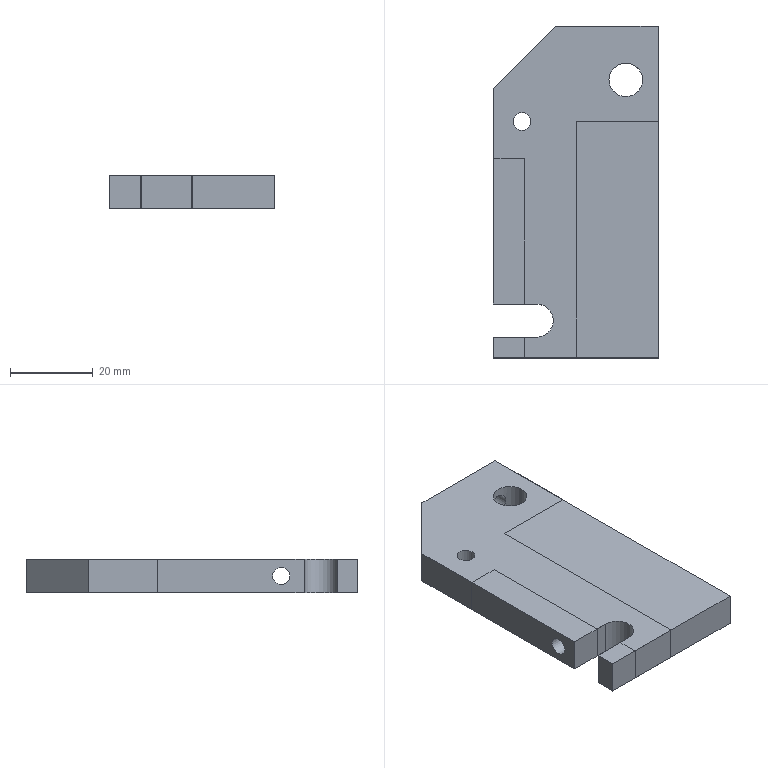NC program | NX | posted with a generic post | part box 40 x 80 x 8 mm
Lines 4877 to 5028 of 5028:
(PLANAR_MILL_COPY , TOOL : D4-12-D4-50-3T-FINISH)
N9722 T11 M6
N9724 G53
N9726 G17 G0 G90 X-27.999 Y11.68 B0. C0. S3000 M3
N9728 G43 Z20. H11
N9730 Z-8.
N9732 G94 G1 Z-10. F300.
N9734 Y10.95
N9736 G3 X-26.999 Y9.95 R1.
N9738 X-24.949 Y12. R2.05
N9740 X-26.999 Y9.95 R-2.05
N9742 X-25.999 Y10.95 R1.
N9744 G1 X-27.999
N9746 G3 X-26.999 Y9.95 R1.
N9748 X-24.949 Y12. R2.05
N9750 X-26.999 Y9.95 R-2.05
N9752 X-25.999 Y10.95 R1.
N9754 G1 Y11.68
N9756 Z-8.
N9758 G0 Z20.
N9760 M5
(DRILLING_1 , TOOL : 上排M5-22-D5.5-60)
N9762 T12 M6
N9764 G53
N9766 G17 G0 G90 X-16.999 Y-13. B0. C0. S300 M3
N9768 G43 Z20. H12
N9770 G84 G94 G99 Z-5. F240. R3.
N9772 G80
N9774 G0 X-16.999 Y-13. Z20.
N9776 M5
(PLANAR_MILL_1 , TOOL : 倒角D4-90度)
N9778 T05 M6
N9780 G53
N9782 G17 G0 G90 X30.322 Y-21.087 B0. C0. S3000 M3
N9784 G43 Z20. H5
N9786 Z1.
N9788 G94 G1 Z-1. F800.
N9790 G41 X29.83 Y-21. D5
N9792 X27.001
N9794 X-24.999
N9796 G2 X-25.706 Y-20.707 R1.
N9798 G1 X-40.706 Y-5.707
N9800 G2 X-40.999 Y-5. R1.
N9802 G1 Y20.
N9804 G2 X-39.999 Y21. R1.
N9806 G1 X40.001
N9808 G2 X41.001 Y20. R1.
N9810 G1 Y-20.
N9812 G2 X40.001 Y-21. R1.
N9814 G1 X35.001
N9816 G2 X34.001 Y-20. R1.
N9818 G1 Y-9.5
N9820 G3 X31.001 Y-6.5 R3.
N9822 X28.001 Y-9.5 R3.
N9824 G1 Y-19.999
N9826 Y-22.828
N9828 G40
N9830 X28.088 Y-23.321
N9832 Z1.
N9834 G0 Z20.
(PLANAR_MILL_2 , TOOL : 倒角D4-90度)
N9836 X-27.912 Y10.703
N9838 Z1.
N9840 G1 Z-1.
N9842 G41 X-27.999 Y10.21
N9844 Y9.95
N9846 G3 X-26.999 Y8.95 R1.
N9848 X-23.949 Y12. R3.05
N9850 X-26.999 Y8.95 R-3.05
N9852 X-25.999 Y9.95 R1.
N9854 G1 Y10.21
N9856 G40
N9858 X-26.086 Y10.703
N9860 Z1.
N9862 G0 Z20.
N9864 M5
(PLANAR_MILL_3 , TOOL : D6-18-D6-50-3T-FINISH)
N9866 T06 M6
N9868 G53
N9870 G17 G0 G90 X0.001 Y26. B0. C0. S3000 M3
N9872 G43 Z20. H6
N9874 Z-7.
N9876 G94 G1 Z-10. F600.
N9878 Y23.
N9880 X40.001
N9882 G2 X43.001 Y20. R3.
N9884 G1 Y-20.
N9886 G2 X40.001 Y-23. R3.
N9888 G1 X35.001
N9890 G2 X32.001 Y-20. R3.
N9892 G1 Y-9.5
N9894 G3 X31.001 Y-8.5 R1.
N9896 X30.001 Y-9.5 R1.
N9898 G1 Y-20.
N9900 G2 X27.001 Y-23. R3.
N9902 G1 X-24.999
N9904 G2 X-27.12 Y-22.121 R3.
N9906 G1 X-42.12 Y-7.121
N9908 G2 X-42.999 Y-5. R3.
N9910 G1 Y20.
N9912 G2 X-39.999 Y23. R3.
N9914 G1 X0.001
N9916 Y26.
N9918 Y23.
N9920 X40.001
N9922 G2 X43.001 Y20. R3.
N9924 G1 Y-20.
N9926 G2 X40.001 Y-23. R3.
N9928 G1 X35.001
N9930 G2 X32.001 Y-20. R3.
N9932 G1 Y-9.5
N9934 G3 X31.001 Y-8.5 R1.
N9936 X30.001 Y-9.5 R1.
N9938 G1 Y-20.
N9940 G2 X27.001 Y-23. R3.
N9942 G1 X-24.999
N9944 G2 X-27.12 Y-22.121 R3.
N9946 G1 X-42.12 Y-7.121
N9948 G2 X-42.999 Y-5. R3.
N9950 G1 Y20.
N9952 G2 X-39.999 Y23. R3.
N9954 G1 X0.001
N9956 Y26.
N9958 Z-7.
N9960 G0 Z20.
N9962 M5
(FLOOR_FACING_1_COPY , TOOL : D63面刀)
N9964 T10 M6
N9966 G53
N9968 G17 G0 G90 X74.501 Y-4.25 B0. C0. S1600 M3
N9970 G43 Z20. H10
N9972 Z3.
N9974 G94 G1 Z0. F600.
N9976 X71.501
N9978 X-71.499
N9980 X-74.499
N9982 Z3.
N9984 G0 Z20.
N9986 M5
N9988 M2